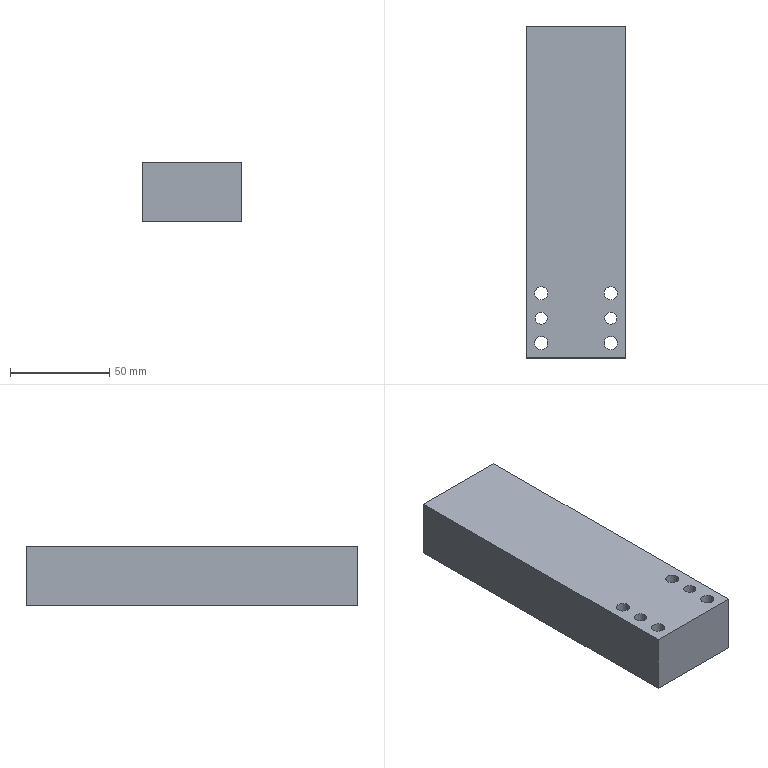Part | NX | features BREP 1 | 1 solid | 28 faces | box 50 x 167 x 30 mm | volume 241820 mm3 | cylinder 14 | plane 10 | cone 4 | commonest cylinder face diameters 6 x4 6.6 x4 11 x4 5 x2
STEP:
#1=CARTESIAN_POINT('',(25.,-83.5,0.));
#2=VERTEX_POINT('',#1);
#3=CARTESIAN_POINT('',(25.,83.5,0.));
#4=VERTEX_POINT('',#3);
#5=CARTESIAN_POINT('',(25.,83.5,0.));
#6=DIRECTION('',(0.,1.,0.));
#7=VECTOR('',#6,1000.);
#8=LINE('',#5,#7);
#9=EDGE_CURVE('',#2,#4,#8,.T.);
#10=ORIENTED_EDGE('',*,*,#9,.T.);
#11=CARTESIAN_POINT('',(25.,83.5,30.));
#12=VERTEX_POINT('',#11);
#13=CARTESIAN_POINT('',(25.,83.5,30.));
#14=DIRECTION('',(0.,0.,-1.));
#15=VECTOR('',#14,1000.);
#16=LINE('',#13,#15);
#17=EDGE_CURVE('',#12,#4,#16,.T.);
#18=ORIENTED_EDGE('',*,*,#17,.F.);
#19=CARTESIAN_POINT('',(25.,-83.5,30.));
#20=VERTEX_POINT('',#19);
#21=CARTESIAN_POINT('',(25.,83.5,30.));
#22=DIRECTION('',(0.,1.,0.));
#23=VECTOR('',#22,1000.);
#24=LINE('',#21,#23);
#25=EDGE_CURVE('',#20,#12,#24,.T.);
#26=ORIENTED_EDGE('',*,*,#25,.F.);
#27=CARTESIAN_POINT('',(25.,-83.5,30.));
#28=DIRECTION('',(0.,0.,-1.));
#29=VECTOR('',#28,1000.);
#30=LINE('',#27,#29);
#31=EDGE_CURVE('',#20,#2,#30,.T.);
#32=ORIENTED_EDGE('',*,*,#31,.T.);
#33=EDGE_LOOP('',(#10,#18,#26,#32));
#34=FACE_BOUND('',#33,.T.);
#35=CARTESIAN_POINT('',(25.,83.5,30.));
#36=DIRECTION('',(-1.,0.,0.));
#37=DIRECTION('',(0.,1.,0.));
#38=AXIS2_PLACEMENT_3D('',#35,#36,#37);
#39=PLANE('',#38);
#40=ADVANCED_FACE('',(#34),#39,.F.);
#41=CARTESIAN_POINT('',(-9.5,83.5,17.5));
#42=VERTEX_POINT('',#41);
#43=CARTESIAN_POINT('',(-9.5,83.5,15.));
#44=DIRECTION('',(0.,1.,0.));
#45=DIRECTION('',(0.,0.,1.));
#46=AXIS2_PLACEMENT_3D('',#43,#44,#45);
#47=CIRCLE('',#46,2.5);
#48=EDGE_CURVE('',#42,#42,#47,.T.);
#49=ORIENTED_EDGE('',*,*,#48,.F.);
#50=EDGE_LOOP('',(#49));
#51=FACE_BOUND('',#50,.T.);
#52=CARTESIAN_POINT('',(9.5,83.5,17.5));
#53=VERTEX_POINT('',#52);
#54=CARTESIAN_POINT('',(9.5,83.5,15.));
#55=DIRECTION('',(0.,1.,0.));
#56=DIRECTION('',(0.,0.,1.));
#57=AXIS2_PLACEMENT_3D('',#54,#55,#56);
#58=CIRCLE('',#57,2.5);
#59=EDGE_CURVE('',#53,#53,#58,.T.);
#60=ORIENTED_EDGE('',*,*,#59,.F.);
#61=EDGE_LOOP('',(#60));
#62=FACE_BOUND('',#61,.T.);
#63=CARTESIAN_POINT('',(-19.,83.5,18.));
#64=VERTEX_POINT('',#63);
#65=CARTESIAN_POINT('',(-19.,83.5,15.));
#66=DIRECTION('',(0.,1.,0.));
#67=DIRECTION('',(0.,0.,1.));
#68=AXIS2_PLACEMENT_3D('',#65,#66,#67);
#69=CIRCLE('',#68,3.);
#70=EDGE_CURVE('',#64,#64,#69,.T.);
#71=ORIENTED_EDGE('',*,*,#70,.F.);
#72=EDGE_LOOP('',(#71));
#73=FACE_BOUND('',#72,.T.);
#74=CARTESIAN_POINT('',(19.,83.5,18.));
#75=VERTEX_POINT('',#74);
#76=CARTESIAN_POINT('',(19.,83.5,15.));
#77=DIRECTION('',(0.,1.,0.));
#78=DIRECTION('',(0.,0.,1.));
#79=AXIS2_PLACEMENT_3D('',#76,#77,#78);
#80=CIRCLE('',#79,3.);
#81=EDGE_CURVE('',#75,#75,#80,.T.);
#82=ORIENTED_EDGE('',*,*,#81,.F.);
#83=EDGE_LOOP('',(#82));
#84=FACE_BOUND('',#83,.T.);
#85=CARTESIAN_POINT('',(-25.,83.5,0.));
#86=VERTEX_POINT('',#85);
#87=CARTESIAN_POINT('',(-25.,83.5,0.));
#88=DIRECTION('',(-1.,0.,0.));
#89=VECTOR('',#88,1000.);
#90=LINE('',#87,#89);
#91=EDGE_CURVE('',#4,#86,#90,.T.);
#92=ORIENTED_EDGE('',*,*,#91,.T.);
#93=CARTESIAN_POINT('',(-25.,83.5,30.));
#94=VERTEX_POINT('',#93);
#95=CARTESIAN_POINT('',(-25.,83.5,30.));
#96=DIRECTION('',(0.,0.,-1.));
#97=VECTOR('',#96,1000.);
#98=LINE('',#95,#97);
#99=EDGE_CURVE('',#94,#86,#98,.T.);
#100=ORIENTED_EDGE('',*,*,#99,.F.);
#101=CARTESIAN_POINT('',(-25.,83.5,30.));
#102=DIRECTION('',(-1.,0.,0.));
#103=VECTOR('',#102,1000.);
#104=LINE('',#101,#103);
#105=EDGE_CURVE('',#12,#94,#104,.T.);
#106=ORIENTED_EDGE('',*,*,#105,.F.);
#107=ORIENTED_EDGE('',*,*,#17,.T.);
#108=EDGE_LOOP('',(#92,#100,#106,#107));
#109=FACE_BOUND('',#108,.T.);
#110=CARTESIAN_POINT('',(-25.,83.5,30.));
#111=DIRECTION('',(0.,-1.,0.));
#112=DIRECTION('',(0.,0.,1.));
#113=AXIS2_PLACEMENT_3D('',#110,#111,#112);
#114=PLANE('',#113);
#115=ADVANCED_FACE('',(#51,#62,#73,#84,#109),#114,.F.);
#116=CARTESIAN_POINT('',(-25.,-83.5,0.));
#117=VERTEX_POINT('',#116);
#118=CARTESIAN_POINT('',(-25.,83.5,0.));
#119=DIRECTION('',(0.,-1.,0.));
#120=VECTOR('',#119,1000.);
#121=LINE('',#118,#120);
#122=EDGE_CURVE('',#86,#117,#121,.T.);
#123=ORIENTED_EDGE('',*,*,#122,.T.);
#124=CARTESIAN_POINT('',(-25.,-83.5,30.));
#125=VERTEX_POINT('',#124);
#126=CARTESIAN_POINT('',(-25.,-83.5,30.));
#127=DIRECTION('',(0.,0.,-1.));
#128=VECTOR('',#127,1000.);
#129=LINE('',#126,#128);
#130=EDGE_CURVE('',#125,#117,#129,.T.);
#131=ORIENTED_EDGE('',*,*,#130,.F.);
#132=CARTESIAN_POINT('',(-25.,83.5,30.));
#133=DIRECTION('',(0.,-1.,0.));
#134=VECTOR('',#133,1000.);
#135=LINE('',#132,#134);
#136=EDGE_CURVE('',#94,#125,#135,.T.);
#137=ORIENTED_EDGE('',*,*,#136,.F.);
#138=ORIENTED_EDGE('',*,*,#99,.T.);
#139=EDGE_LOOP('',(#123,#131,#137,#138));
#140=FACE_BOUND('',#139,.T.);
#141=CARTESIAN_POINT('',(-25.,83.5,30.));
#142=DIRECTION('',(1.,0.,0.));
#143=DIRECTION('',(0.,-1.,0.));
#144=AXIS2_PLACEMENT_3D('',#141,#142,#143);
#145=PLANE('',#144);
#146=ADVANCED_FACE('',(#140),#145,.F.);
#147=CARTESIAN_POINT('',(-25.,-83.5,0.));
#148=DIRECTION('',(1.,0.,0.));
#149=VECTOR('',#148,1000.);
#150=LINE('',#147,#149);
#151=EDGE_CURVE('',#117,#2,#150,.T.);
#152=ORIENTED_EDGE('',*,*,#151,.T.);
#153=ORIENTED_EDGE('',*,*,#31,.F.);
#154=CARTESIAN_POINT('',(-25.,-83.5,30.));
#155=DIRECTION('',(1.,0.,0.));
#156=VECTOR('',#155,1000.);
#157=LINE('',#154,#156);
#158=EDGE_CURVE('',#125,#20,#157,.T.);
#159=ORIENTED_EDGE('',*,*,#158,.F.);
#160=ORIENTED_EDGE('',*,*,#130,.T.);
#161=EDGE_LOOP('',(#152,#153,#159,#160));
#162=FACE_BOUND('',#161,.T.);
#163=CARTESIAN_POINT('',(-25.,-83.5,30.));
#164=DIRECTION('',(0.,1.,0.));
#165=DIRECTION('',(0.,0.,-1.));
#166=AXIS2_PLACEMENT_3D('',#163,#164,#165);
#167=PLANE('',#166);
#168=ADVANCED_FACE('',(#162),#167,.F.);
#169=CARTESIAN_POINT('',(14.2,-76.,30.));
#170=VERTEX_POINT('',#169);
#171=CARTESIAN_POINT('',(17.5,-76.,30.));
#172=DIRECTION('',(0.,0.,-1.));
#173=DIRECTION('',(-1.,0.,0.));
#174=AXIS2_PLACEMENT_3D('',#171,#172,#173);
#175=CIRCLE('',#174,3.3);
#176=EDGE_CURVE('',#170,#170,#175,.T.);
#177=ORIENTED_EDGE('',*,*,#176,.T.);
#178=EDGE_LOOP('',(#177));
#179=FACE_BOUND('',#178,.T.);
#180=CARTESIAN_POINT('',(14.2,-51.,30.));
#181=VERTEX_POINT('',#180);
#182=CARTESIAN_POINT('',(17.5,-51.,30.));
#183=DIRECTION('',(0.,0.,-1.));
#184=DIRECTION('',(-1.,0.,0.));
#185=AXIS2_PLACEMENT_3D('',#182,#183,#184);
#186=CIRCLE('',#185,3.3);
#187=EDGE_CURVE('',#181,#181,#186,.T.);
#188=ORIENTED_EDGE('',*,*,#187,.T.);
#189=EDGE_LOOP('',(#188));
#190=FACE_BOUND('',#189,.T.);
#191=CARTESIAN_POINT('',(-20.8,-76.,30.));
#192=VERTEX_POINT('',#191);
#193=CARTESIAN_POINT('',(-17.5,-76.,30.));
#194=DIRECTION('',(0.,0.,-1.));
#195=DIRECTION('',(-1.,0.,0.));
#196=AXIS2_PLACEMENT_3D('',#193,#194,#195);
#197=CIRCLE('',#196,3.3);
#198=EDGE_CURVE('',#192,#192,#197,.T.);
#199=ORIENTED_EDGE('',*,*,#198,.T.);
#200=EDGE_LOOP('',(#199));
#201=FACE_BOUND('',#200,.T.);
#202=CARTESIAN_POINT('',(-20.8,-51.,30.));
#203=VERTEX_POINT('',#202);
#204=CARTESIAN_POINT('',(-17.5,-51.,30.));
#205=DIRECTION('',(0.,0.,-1.));
#206=DIRECTION('',(-1.,0.,0.));
#207=AXIS2_PLACEMENT_3D('',#204,#205,#206);
#208=CIRCLE('',#207,3.3);
#209=EDGE_CURVE('',#203,#203,#208,.T.);
#210=ORIENTED_EDGE('',*,*,#209,.T.);
#211=EDGE_LOOP('',(#210));
#212=FACE_BOUND('',#211,.T.);
#213=CARTESIAN_POINT('',(14.5,-63.5,30.));
#214=VERTEX_POINT('',#213);
#215=CARTESIAN_POINT('',(17.5,-63.5,30.));
#216=DIRECTION('',(0.,0.,-1.));
#217=DIRECTION('',(-1.,0.,0.));
#218=AXIS2_PLACEMENT_3D('',#215,#216,#217);
#219=CIRCLE('',#218,3.);
#220=EDGE_CURVE('',#214,#214,#219,.T.);
#221=ORIENTED_EDGE('',*,*,#220,.T.);
#222=EDGE_LOOP('',(#221));
#223=FACE_BOUND('',#222,.T.);
#224=CARTESIAN_POINT('',(-20.5,-63.5,30.));
#225=VERTEX_POINT('',#224);
#226=CARTESIAN_POINT('',(-17.5,-63.5,30.));
#227=DIRECTION('',(0.,0.,-1.));
#228=DIRECTION('',(-1.,0.,0.));
#229=AXIS2_PLACEMENT_3D('',#226,#227,#228);
#230=CIRCLE('',#229,3.);
#231=EDGE_CURVE('',#225,#225,#230,.T.);
#232=ORIENTED_EDGE('',*,*,#231,.T.);
#233=EDGE_LOOP('',(#232));
#234=FACE_BOUND('',#233,.T.);
#235=ORIENTED_EDGE('',*,*,#25,.T.);
#236=ORIENTED_EDGE('',*,*,#105,.T.);
#237=ORIENTED_EDGE('',*,*,#136,.T.);
#238=ORIENTED_EDGE('',*,*,#158,.T.);
#239=EDGE_LOOP('',(#235,#236,#237,#238));
#240=FACE_BOUND('',#239,.T.);
#241=CARTESIAN_POINT('',(0.,0.,30.));
#242=DIRECTION('',(0.,0.,1.));
#243=DIRECTION('',(-1.,0.,0.));
#244=AXIS2_PLACEMENT_3D('',#241,#242,#243);
#245=PLANE('',#244);
#246=ADVANCED_FACE('',(#179,#190,#201,#212,#223,#234,#240),#245,.T.);
#247=CARTESIAN_POINT('',(12.,-76.,0.));
#248=VERTEX_POINT('',#247);
#249=CARTESIAN_POINT('',(17.5,-76.,0.));
#250=DIRECTION('',(0.,0.,-1.));
#251=DIRECTION('',(-1.,0.,0.));
#252=AXIS2_PLACEMENT_3D('',#249,#250,#251);
#253=CIRCLE('',#252,5.5);
#254=EDGE_CURVE('',#248,#248,#253,.T.);
#255=ORIENTED_EDGE('',*,*,#254,.F.);
#256=EDGE_LOOP('',(#255));
#257=FACE_BOUND('',#256,.T.);
#258=CARTESIAN_POINT('',(12.,-51.,0.));
#259=VERTEX_POINT('',#258);
#260=CARTESIAN_POINT('',(17.5,-51.,0.));
#261=DIRECTION('',(0.,0.,-1.));
#262=DIRECTION('',(-1.,0.,0.));
#263=AXIS2_PLACEMENT_3D('',#260,#261,#262);
#264=CIRCLE('',#263,5.5);
#265=EDGE_CURVE('',#259,#259,#264,.T.);
#266=ORIENTED_EDGE('',*,*,#265,.F.);
#267=EDGE_LOOP('',(#266));
#268=FACE_BOUND('',#267,.T.);
#269=CARTESIAN_POINT('',(-23.,-76.,0.));
#270=VERTEX_POINT('',#269);
#271=CARTESIAN_POINT('',(-17.5,-76.,0.));
#272=DIRECTION('',(0.,0.,-1.));
#273=DIRECTION('',(-1.,0.,0.));
#274=AXIS2_PLACEMENT_3D('',#271,#272,#273);
#275=CIRCLE('',#274,5.5);
#276=EDGE_CURVE('',#270,#270,#275,.T.);
#277=ORIENTED_EDGE('',*,*,#276,.F.);
#278=EDGE_LOOP('',(#277));
#279=FACE_BOUND('',#278,.T.);
#280=CARTESIAN_POINT('',(-23.,-51.,0.));
#281=VERTEX_POINT('',#280);
#282=CARTESIAN_POINT('',(-17.5,-51.,0.));
#283=DIRECTION('',(0.,0.,-1.));
#284=DIRECTION('',(-1.,0.,0.));
#285=AXIS2_PLACEMENT_3D('',#282,#283,#284);
#286=CIRCLE('',#285,5.5);
#287=EDGE_CURVE('',#281,#281,#286,.T.);
#288=ORIENTED_EDGE('',*,*,#287,.F.);
#289=EDGE_LOOP('',(#288));
#290=FACE_BOUND('',#289,.T.);
#291=CARTESIAN_POINT('',(14.5,-63.5,0.));
#292=VERTEX_POINT('',#291);
#293=CARTESIAN_POINT('',(17.5,-63.5,0.));
#294=DIRECTION('',(0.,0.,-1.));
#295=DIRECTION('',(-1.,0.,0.));
#296=AXIS2_PLACEMENT_3D('',#293,#294,#295);
#297=CIRCLE('',#296,3.);
#298=EDGE_CURVE('',#292,#292,#297,.T.);
#299=ORIENTED_EDGE('',*,*,#298,.F.);
#300=EDGE_LOOP('',(#299));
#301=FACE_BOUND('',#300,.T.);
#302=CARTESIAN_POINT('',(-20.5,-63.5,0.));
#303=VERTEX_POINT('',#302);
#304=CARTESIAN_POINT('',(-17.5,-63.5,0.));
#305=DIRECTION('',(0.,0.,-1.));
#306=DIRECTION('',(-1.,0.,0.));
#307=AXIS2_PLACEMENT_3D('',#304,#305,#306);
#308=CIRCLE('',#307,3.);
#309=EDGE_CURVE('',#303,#303,#308,.T.);
#310=ORIENTED_EDGE('',*,*,#309,.F.);
#311=EDGE_LOOP('',(#310));
#312=FACE_BOUND('',#311,.T.);
#313=ORIENTED_EDGE('',*,*,#9,.F.);
#314=ORIENTED_EDGE('',*,*,#151,.F.);
#315=ORIENTED_EDGE('',*,*,#122,.F.);
#316=ORIENTED_EDGE('',*,*,#91,.F.);
#317=EDGE_LOOP('',(#313,#314,#315,#316));
#318=FACE_BOUND('',#317,.T.);
#319=CARTESIAN_POINT('',(0.,0.,0.));
#320=DIRECTION('',(0.,0.,1.));
#321=DIRECTION('',(-1.,0.,0.));
#322=AXIS2_PLACEMENT_3D('',#319,#320,#321);
#323=PLANE('',#322);
#324=ADVANCED_FACE('',(#257,#268,#279,#290,#301,#312,#318),#323,.F.);
#325=ORIENTED_EDGE('',*,*,#231,.F.);
#326=EDGE_LOOP('',(#325));
#327=FACE_BOUND('',#326,.T.);
#328=ORIENTED_EDGE('',*,*,#309,.T.);
#329=EDGE_LOOP('',(#328));
#330=FACE_BOUND('',#329,.T.);
#331=CARTESIAN_POINT('',(-17.5,-63.5,0.));
#332=DIRECTION('',(0.,0.,-1.));
#333=DIRECTION('',(1.,0.,0.));
#334=AXIS2_PLACEMENT_3D('',#331,#332,#333);
#335=CYLINDRICAL_SURFACE('',#334,3.);
#336=ADVANCED_FACE('',(#327,#330),#335,.F.);
#337=ORIENTED_EDGE('',*,*,#220,.F.);
#338=EDGE_LOOP('',(#337));
#339=FACE_BOUND('',#338,.T.);
#340=ORIENTED_EDGE('',*,*,#298,.T.);
#341=EDGE_LOOP('',(#340));
#342=FACE_BOUND('',#341,.T.);
#343=CARTESIAN_POINT('',(17.5,-63.5,0.));
#344=DIRECTION('',(0.,0.,-1.));
#345=DIRECTION('',(1.,0.,0.));
#346=AXIS2_PLACEMENT_3D('',#343,#344,#345);
#347=CYLINDRICAL_SURFACE('',#346,3.);
#348=ADVANCED_FACE('',(#339,#342),#347,.F.);
#349=ORIENTED_EDGE('',*,*,#209,.F.);
#350=EDGE_LOOP('',(#349));
#351=FACE_BOUND('',#350,.T.);
#352=CARTESIAN_POINT('',(-20.8,-51.,6.4));
#353=VERTEX_POINT('',#352);
#354=CARTESIAN_POINT('',(-17.5,-51.,6.4));
#355=DIRECTION('',(0.,0.,-1.));
#356=DIRECTION('',(-1.,0.,0.));
#357=AXIS2_PLACEMENT_3D('',#354,#355,#356);
#358=CIRCLE('',#357,3.3);
#359=EDGE_CURVE('',#353,#353,#358,.T.);
#360=ORIENTED_EDGE('',*,*,#359,.T.);
#361=EDGE_LOOP('',(#360));
#362=FACE_BOUND('',#361,.T.);
#363=CARTESIAN_POINT('',(-17.5,-51.,0.));
#364=DIRECTION('',(0.,0.,-1.));
#365=DIRECTION('',(1.,0.,0.));
#366=AXIS2_PLACEMENT_3D('',#363,#364,#365);
#367=CYLINDRICAL_SURFACE('',#366,3.3);
#368=ADVANCED_FACE('',(#351,#362),#367,.F.);
#369=ORIENTED_EDGE('',*,*,#359,.F.);
#370=EDGE_LOOP('',(#369));
#371=FACE_BOUND('',#370,.T.);
#372=CARTESIAN_POINT('',(-23.,-51.,6.4));
#373=VERTEX_POINT('',#372);
#374=CARTESIAN_POINT('',(-17.5,-51.,6.4));
#375=DIRECTION('',(0.,0.,-1.));
#376=DIRECTION('',(-1.,0.,0.));
#377=AXIS2_PLACEMENT_3D('',#374,#375,#376);
#378=CIRCLE('',#377,5.5);
#379=EDGE_CURVE('',#373,#373,#378,.T.);
#380=ORIENTED_EDGE('',*,*,#379,.T.);
#381=EDGE_LOOP('',(#380));
#382=FACE_BOUND('',#381,.T.);
#383=CARTESIAN_POINT('',(-14.2,-51.,6.4));
#384=DIRECTION('',(0.,0.,1.));
#385=DIRECTION('',(-1.,0.,0.));
#386=AXIS2_PLACEMENT_3D('',#383,#384,#385);
#387=PLANE('',#386);
#388=ADVANCED_FACE('',(#371,#382),#387,.F.);
#389=ORIENTED_EDGE('',*,*,#379,.F.);
#390=EDGE_LOOP('',(#389));
#391=FACE_BOUND('',#390,.T.);
#392=ORIENTED_EDGE('',*,*,#287,.T.);
#393=EDGE_LOOP('',(#392));
#394=FACE_BOUND('',#393,.T.);
#395=CARTESIAN_POINT('',(-17.5,-51.,0.));
#396=DIRECTION('',(0.,0.,-1.));
#397=DIRECTION('',(1.,0.,0.));
#398=AXIS2_PLACEMENT_3D('',#395,#396,#397);
#399=CYLINDRICAL_SURFACE('',#398,5.5);
#400=ADVANCED_FACE('',(#391,#394),#399,.F.);
#401=ORIENTED_EDGE('',*,*,#198,.F.);
#402=EDGE_LOOP('',(#401));
#403=FACE_BOUND('',#402,.T.);
#404=CARTESIAN_POINT('',(-20.8,-76.,6.4));
#405=VERTEX_POINT('',#404);
#406=CARTESIAN_POINT('',(-17.5,-76.,6.4));
#407=DIRECTION('',(0.,0.,-1.));
#408=DIRECTION('',(-1.,0.,0.));
#409=AXIS2_PLACEMENT_3D('',#406,#407,#408);
#410=CIRCLE('',#409,3.3);
#411=EDGE_CURVE('',#405,#405,#410,.T.);
#412=ORIENTED_EDGE('',*,*,#411,.T.);
#413=EDGE_LOOP('',(#412));
#414=FACE_BOUND('',#413,.T.);
#415=CARTESIAN_POINT('',(-17.5,-76.,0.));
#416=DIRECTION('',(0.,0.,-1.));
#417=DIRECTION('',(1.,0.,0.));
#418=AXIS2_PLACEMENT_3D('',#415,#416,#417);
#419=CYLINDRICAL_SURFACE('',#418,3.3);
#420=ADVANCED_FACE('',(#403,#414),#419,.F.);
#421=ORIENTED_EDGE('',*,*,#411,.F.);
#422=EDGE_LOOP('',(#421));
#423=FACE_BOUND('',#422,.T.);
#424=CARTESIAN_POINT('',(-23.,-76.,6.4));
#425=VERTEX_POINT('',#424);
#426=CARTESIAN_POINT('',(-17.5,-76.,6.4));
#427=DIRECTION('',(0.,0.,-1.));
#428=DIRECTION('',(-1.,0.,0.));
#429=AXIS2_PLACEMENT_3D('',#426,#427,#428);
#430=CIRCLE('',#429,5.5);
#431=EDGE_CURVE('',#425,#425,#430,.T.);
#432=ORIENTED_EDGE('',*,*,#431,.T.);
#433=EDGE_LOOP('',(#432));
#434=FACE_BOUND('',#433,.T.);
#435=CARTESIAN_POINT('',(-14.2,-76.,6.4));
#436=DIRECTION('',(0.,0.,1.));
#437=DIRECTION('',(-1.,0.,0.));
#438=AXIS2_PLACEMENT_3D('',#435,#436,#437);
#439=PLANE('',#438);
#440=ADVANCED_FACE('',(#423,#434),#439,.F.);
#441=ORIENTED_EDGE('',*,*,#431,.F.);
#442=EDGE_LOOP('',(#441));
#443=FACE_BOUND('',#442,.T.);
#444=ORIENTED_EDGE('',*,*,#276,.T.);
#445=EDGE_LOOP('',(#444));
#446=FACE_BOUND('',#445,.T.);
#447=CARTESIAN_POINT('',(-17.5,-76.,0.));
#448=DIRECTION('',(0.,0.,-1.));
#449=DIRECTION('',(1.,0.,0.));
#450=AXIS2_PLACEMENT_3D('',#447,#448,#449);
#451=CYLINDRICAL_SURFACE('',#450,5.5);
#452=ADVANCED_FACE('',(#443,#446),#451,.F.);
#453=ORIENTED_EDGE('',*,*,#187,.F.);
#454=EDGE_LOOP('',(#453));
#455=FACE_BOUND('',#454,.T.);
#456=CARTESIAN_POINT('',(14.2,-51.,6.4));
#457=VERTEX_POINT('',#456);
#458=CARTESIAN_POINT('',(17.5,-51.,6.4));
#459=DIRECTION('',(0.,0.,-1.));
#460=DIRECTION('',(-1.,0.,0.));
#461=AXIS2_PLACEMENT_3D('',#458,#459,#460);
#462=CIRCLE('',#461,3.3);
#463=EDGE_CURVE('',#457,#457,#462,.T.);
#464=ORIENTED_EDGE('',*,*,#463,.T.);
#465=EDGE_LOOP('',(#464));
#466=FACE_BOUND('',#465,.T.);
#467=CARTESIAN_POINT('',(17.5,-51.,0.));
#468=DIRECTION('',(0.,0.,-1.));
#469=DIRECTION('',(1.,0.,0.));
#470=AXIS2_PLACEMENT_3D('',#467,#468,#469);
#471=CYLINDRICAL_SURFACE('',#470,3.3);
#472=ADVANCED_FACE('',(#455,#466),#471,.F.);
#473=ORIENTED_EDGE('',*,*,#463,.F.);
#474=EDGE_LOOP('',(#473));
#475=FACE_BOUND('',#474,.T.);
#476=CARTESIAN_POINT('',(12.,-51.,6.4));
#477=VERTEX_POINT('',#476);
#478=CARTESIAN_POINT('',(17.5,-51.,6.4));
#479=DIRECTION('',(0.,0.,-1.));
#480=DIRECTION('',(-1.,0.,0.));
#481=AXIS2_PLACEMENT_3D('',#478,#479,#480);
#482=CIRCLE('',#481,5.5);
#483=EDGE_CURVE('',#477,#477,#482,.T.);
#484=ORIENTED_EDGE('',*,*,#483,.T.);
#485=EDGE_LOOP('',(#484));
#486=FACE_BOUND('',#485,.T.);
#487=CARTESIAN_POINT('',(20.8,-51.,6.4));
#488=DIRECTION('',(0.,0.,1.));
#489=DIRECTION('',(-1.,0.,0.));
#490=AXIS2_PLACEMENT_3D('',#487,#488,#489);
#491=PLANE('',#490);
#492=ADVANCED_FACE('',(#475,#486),#491,.F.);
#493=ORIENTED_EDGE('',*,*,#483,.F.);
#494=EDGE_LOOP('',(#493));
#495=FACE_BOUND('',#494,.T.);
#496=ORIENTED_EDGE('',*,*,#265,.T.);
#497=EDGE_LOOP('',(#496));
#498=FACE_BOUND('',#497,.T.);
#499=CARTESIAN_POINT('',(17.5,-51.,0.));
#500=DIRECTION('',(0.,0.,-1.));
#501=DIRECTION('',(1.,0.,0.));
#502=AXIS2_PLACEMENT_3D('',#499,#500,#501);
#503=CYLINDRICAL_SURFACE('',#502,5.5);
#504=ADVANCED_FACE('',(#495,#498),#503,.F.);
#505=ORIENTED_EDGE('',*,*,#176,.F.);
#506=EDGE_LOOP('',(#505));
#507=FACE_BOUND('',#506,.T.);
#508=CARTESIAN_POINT('',(14.2,-76.,6.4));
#509=VERTEX_POINT('',#508);
#510=CARTESIAN_POINT('',(17.5,-76.,6.4));
#511=DIRECTION('',(0.,0.,-1.));
#512=DIRECTION('',(-1.,0.,0.));
#513=AXIS2_PLACEMENT_3D('',#510,#511,#512);
#514=CIRCLE('',#513,3.3);
#515=EDGE_CURVE('',#509,#509,#514,.T.);
#516=ORIENTED_EDGE('',*,*,#515,.T.);
#517=EDGE_LOOP('',(#516));
#518=FACE_BOUND('',#517,.T.);
#519=CARTESIAN_POINT('',(17.5,-76.,0.));
#520=DIRECTION('',(0.,0.,-1.));
#521=DIRECTION('',(1.,0.,0.));
#522=AXIS2_PLACEMENT_3D('',#519,#520,#521);
#523=CYLINDRICAL_SURFACE('',#522,3.3);
#524=ADVANCED_FACE('',(#507,#518),#523,.F.);
#525=ORIENTED_EDGE('',*,*,#515,.F.);
#526=EDGE_LOOP('',(#525));
#527=FACE_BOUND('',#526,.T.);
#528=CARTESIAN_POINT('',(12.,-76.,6.4));
#529=VERTEX_POINT('',#528);
#530=CARTESIAN_POINT('',(17.5,-76.,6.4));
#531=DIRECTION('',(0.,0.,-1.));
#532=DIRECTION('',(-1.,0.,0.));
#533=AXIS2_PLACEMENT_3D('',#530,#531,#532);
#534=CIRCLE('',#533,5.5);
#535=EDGE_CURVE('',#529,#529,#534,.T.);
#536=ORIENTED_EDGE('',*,*,#535,.T.);
#537=EDGE_LOOP('',(#536));
#538=FACE_BOUND('',#537,.T.);
#539=CARTESIAN_POINT('',(20.8,-76.,6.4));
#540=DIRECTION('',(0.,0.,1.));
#541=DIRECTION('',(-1.,0.,0.));
#542=AXIS2_PLACEMENT_3D('',#539,#540,#541);
#543=PLANE('',#542);
#544=ADVANCED_FACE('',(#527,#538),#543,.F.);
#545=ORIENTED_EDGE('',*,*,#535,.F.);
#546=EDGE_LOOP('',(#545));
#547=FACE_BOUND('',#546,.T.);
#548=ORIENTED_EDGE('',*,*,#254,.T.);
#549=EDGE_LOOP('',(#548));
#550=FACE_BOUND('',#549,.T.);
#551=CARTESIAN_POINT('',(17.5,-76.,0.));
#552=DIRECTION('',(0.,0.,-1.));
#553=DIRECTION('',(1.,0.,0.));
#554=AXIS2_PLACEMENT_3D('',#551,#552,#553);
#555=CYLINDRICAL_SURFACE('',#554,5.5);
#556=ADVANCED_FACE('',(#547,#550),#555,.F.);
#557=CARTESIAN_POINT('',(19.,69.697,15.));
#558=VERTEX_POINT('',#557);
#559=VERTEX_LOOP('',#558);
#560=FACE_BOUND('',#559,.T.);
#561=CARTESIAN_POINT('',(19.,71.5,18.));
#562=VERTEX_POINT('',#561);
#563=CARTESIAN_POINT('',(19.,71.5,15.));
#564=DIRECTION('',(0.,1.,0.));
#565=DIRECTION('',(0.,0.,1.));
#566=AXIS2_PLACEMENT_3D('',#563,#564,#565);
#567=CIRCLE('',#566,3.);
#568=EDGE_CURVE('',#562,#562,#567,.T.);
#569=ORIENTED_EDGE('',*,*,#568,.T.);
#570=EDGE_LOOP('',(#569));
#571=FACE_BOUND('',#570,.T.);
#572=CARTESIAN_POINT('',(19.,71.5,15.));
#573=DIRECTION('',(0.,1.,0.));
#574=DIRECTION('',(0.,0.,-1.));
#575=AXIS2_PLACEMENT_3D('',#572,#573,#574);
#576=CONICAL_SURFACE('',#575,3.,1.03);
#577=ADVANCED_FACE('',(#560,#571),#576,.F.);
#578=ORIENTED_EDGE('',*,*,#568,.F.);
#579=EDGE_LOOP('',(#578));
#580=FACE_BOUND('',#579,.T.);
#581=ORIENTED_EDGE('',*,*,#81,.T.);
#582=EDGE_LOOP('',(#581));
#583=FACE_BOUND('',#582,.T.);
#584=CARTESIAN_POINT('',(19.,83.5,15.));
#585=DIRECTION('',(0.,1.,0.));
#586=DIRECTION('',(0.,0.,-1.));
#587=AXIS2_PLACEMENT_3D('',#584,#585,#586);
#588=CYLINDRICAL_SURFACE('',#587,3.);
#589=ADVANCED_FACE('',(#580,#583),#588,.F.);
#590=CARTESIAN_POINT('',(-19.,69.697,15.));
#591=VERTEX_POINT('',#590);
#592=VERTEX_LOOP('',#591);
#593=FACE_BOUND('',#592,.T.);
#594=CARTESIAN_POINT('',(-19.,71.5,18.));
#595=VERTEX_POINT('',#594);
#596=CARTESIAN_POINT('',(-19.,71.5,15.));
#597=DIRECTION('',(0.,1.,0.));
#598=DIRECTION('',(0.,0.,1.));
#599=AXIS2_PLACEMENT_3D('',#596,#597,#598);
#600=CIRCLE('',#599,3.);
#601=EDGE_CURVE('',#595,#595,#600,.T.);
#602=ORIENTED_EDGE('',*,*,#601,.T.);
#603=EDGE_LOOP('',(#602));
#604=FACE_BOUND('',#603,.T.);
#605=CARTESIAN_POINT('',(-19.,71.5,15.));
#606=DIRECTION('',(0.,1.,0.));
#607=DIRECTION('',(0.,0.,-1.));
#608=AXIS2_PLACEMENT_3D('',#605,#606,#607);
#609=CONICAL_SURFACE('',#608,3.,1.03);
#610=ADVANCED_FACE('',(#593,#604),#609,.F.);
#611=ORIENTED_EDGE('',*,*,#601,.F.);
#612=EDGE_LOOP('',(#611));
#613=FACE_BOUND('',#612,.T.);
#614=ORIENTED_EDGE('',*,*,#70,.T.);
#615=EDGE_LOOP('',(#614));
#616=FACE_BOUND('',#615,.T.);
#617=CARTESIAN_POINT('',(-19.,83.5,15.));
#618=DIRECTION('',(0.,1.,0.));
#619=DIRECTION('',(0.,0.,-1.));
#620=AXIS2_PLACEMENT_3D('',#617,#618,#619);
#621=CYLINDRICAL_SURFACE('',#620,3.);
#622=ADVANCED_FACE('',(#613,#616),#621,.F.);
#623=CARTESIAN_POINT('',(9.5,66.998,15.));
#624=VERTEX_POINT('',#623);
#625=VERTEX_LOOP('',#624);
#626=FACE_BOUND('',#625,.T.);
#627=CARTESIAN_POINT('',(9.5,68.5,17.5));
#628=VERTEX_POINT('',#627);
#629=CARTESIAN_POINT('',(9.5,68.5,15.));
#630=DIRECTION('',(0.,1.,0.));
#631=DIRECTION('',(0.,0.,1.));
#632=AXIS2_PLACEMENT_3D('',#629,#630,#631);
#633=CIRCLE('',#632,2.5);
#634=EDGE_CURVE('',#628,#628,#633,.T.);
#635=ORIENTED_EDGE('',*,*,#634,.T.);
#636=EDGE_LOOP('',(#635));
#637=FACE_BOUND('',#636,.T.);
#638=CARTESIAN_POINT('',(9.5,68.5,15.));
#639=DIRECTION('',(0.,1.,0.));
#640=DIRECTION('',(0.,0.,-1.));
#641=AXIS2_PLACEMENT_3D('',#638,#639,#640);
#642=CONICAL_SURFACE('',#641,2.5,1.03);
#643=ADVANCED_FACE('',(#626,#637),#642,.F.);
#644=ORIENTED_EDGE('',*,*,#634,.F.);
#645=EDGE_LOOP('',(#644));
#646=FACE_BOUND('',#645,.T.);
#647=ORIENTED_EDGE('',*,*,#59,.T.);
#648=EDGE_LOOP('',(#647));
#649=FACE_BOUND('',#648,.T.);
#650=CARTESIAN_POINT('',(9.5,83.5,15.));
#651=DIRECTION('',(0.,1.,0.));
#652=DIRECTION('',(0.,0.,-1.));
#653=AXIS2_PLACEMENT_3D('',#650,#651,#652);
#654=CYLINDRICAL_SURFACE('',#653,2.5);
#655=ADVANCED_FACE('',(#646,#649),#654,.F.);
#656=CARTESIAN_POINT('',(-9.5,66.998,15.));
#657=VERTEX_POINT('',#656);
#658=VERTEX_LOOP('',#657);
#659=FACE_BOUND('',#658,.T.);
#660=CARTESIAN_POINT('',(-9.5,68.5,17.5));
#661=VERTEX_POINT('',#660);
#662=CARTESIAN_POINT('',(-9.5,68.5,15.));
#663=DIRECTION('',(0.,1.,0.));
#664=DIRECTION('',(0.,0.,1.));
#665=AXIS2_PLACEMENT_3D('',#662,#663,#664);
#666=CIRCLE('',#665,2.5);
#667=EDGE_CURVE('',#661,#661,#666,.T.);
#668=ORIENTED_EDGE('',*,*,#667,.T.);
#669=EDGE_LOOP('',(#668));
#670=FACE_BOUND('',#669,.T.);
#671=CARTESIAN_POINT('',(-9.5,68.5,15.));
#672=DIRECTION('',(0.,1.,0.));
#673=DIRECTION('',(0.,0.,-1.));
#674=AXIS2_PLACEMENT_3D('',#671,#672,#673);
#675=CONICAL_SURFACE('',#674,2.5,1.03);
#676=ADVANCED_FACE('',(#659,#670),#675,.F.);
#677=ORIENTED_EDGE('',*,*,#667,.F.);
#678=EDGE_LOOP('',(#677));
#679=FACE_BOUND('',#678,.T.);
#680=ORIENTED_EDGE('',*,*,#48,.T.);
#681=EDGE_LOOP('',(#680));
#682=FACE_BOUND('',#681,.T.);
#683=CARTESIAN_POINT('',(-9.5,83.5,15.));
#684=DIRECTION('',(0.,1.,0.));
#685=DIRECTION('',(0.,0.,-1.));
#686=AXIS2_PLACEMENT_3D('',#683,#684,#685);
#687=CYLINDRICAL_SURFACE('',#686,2.5);
#688=ADVANCED_FACE('',(#679,#682),#687,.F.);
#689=CLOSED_SHELL('',(#40,#115,#146,#168,#246,#324,#336,#348,#368,#388,#400,#420,#440,#452,#472,#492,#504,#524,#544,#556,#577,#589,#610,#622,#643,#655,#676,#688));
#690=MANIFOLD_SOLID_BREP('',#689);
#691=(LENGTH_UNIT()NAMED_UNIT(*)SI_UNIT(.MILLI.,.METRE.));
#692=UNCERTAINTY_MEASURE_WITH_UNIT(LENGTH_MEASURE(0.00001),#691,'','');
#693=(NAMED_UNIT(*)PLANE_ANGLE_UNIT()SI_UNIT($,.RADIAN.));
#694=(NAMED_UNIT(*)SI_UNIT($,.STERADIAN.)SOLID_ANGLE_UNIT());
#695=(GEOMETRIC_REPRESENTATION_CONTEXT(3)GLOBAL_UNCERTAINTY_ASSIGNED_CONTEXT((#692))GLOBAL_UNIT_ASSIGNED_CONTEXT((#691,#693,#694))REPRESENTATION_CONTEXT('',''));
#696=ADVANCED_BREP_SHAPE_REPRESENTATION('',(#690),#695);